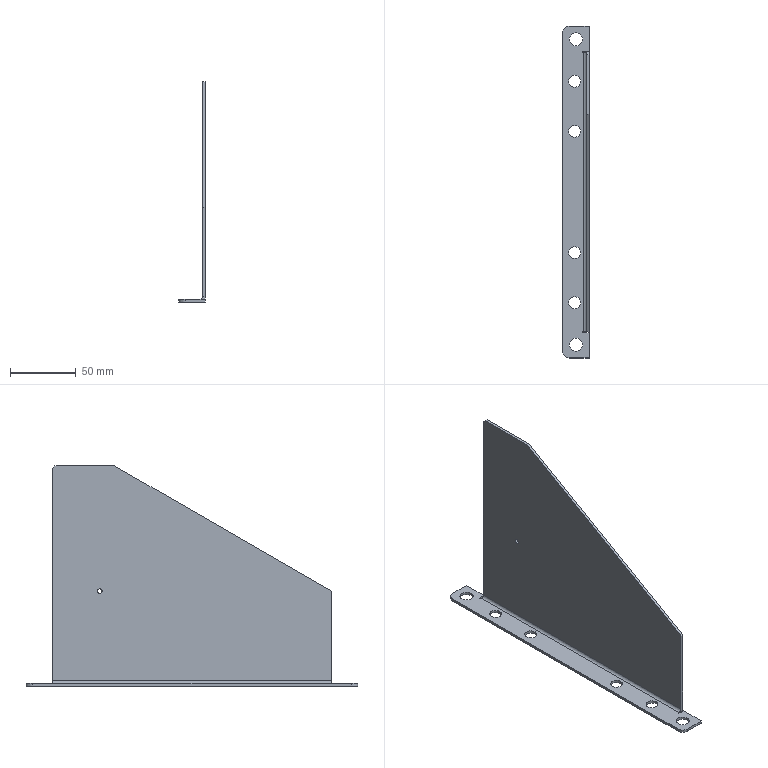Part | STEP file | SYL0380DJ1008_2_7_2_1-3_STEP | 1 solid | 40 faces | box 20 x 252 x 167 mm | volume 62974 mm3 | plane 22 | cylinder 18 | commonest cylinder face diameters 9 x8 10 x6 3.5 x2 4 x1 8 x1
STEP:
#1=CARTESIAN_POINT('',(10.,70.,71.75));
#2=VERTEX_POINT('',#1);
#3=CARTESIAN_POINT('',(8.,70.,71.75));
#4=VERTEX_POINT('',#3);
#5=CARTESIAN_POINT('',(8.,70.,71.75));
#6=DIRECTION('',(-1.,0.,0.));
#7=VECTOR('',#6,1000.);
#8=LINE('',#5,#7);
#9=EDGE_CURVE('',#2,#4,#8,.T.);
#10=ORIENTED_EDGE('',*,*,#9,.F.);
#11=CARTESIAN_POINT('',(10.,70.,68.25));
#12=VERTEX_POINT('',#11);
#13=CARTESIAN_POINT('',(10.,70.,70.));
#14=DIRECTION('',(1.,0.,0.));
#15=DIRECTION('',(0.,0.,-1.));
#16=AXIS2_PLACEMENT_3D('',#13,#14,#15);
#17=CIRCLE('',#16,1.75);
#18=EDGE_CURVE('',#2,#12,#17,.T.);
#19=ORIENTED_EDGE('',*,*,#18,.T.);
#20=CARTESIAN_POINT('',(8.,70.,68.25));
#21=VERTEX_POINT('',#20);
#22=CARTESIAN_POINT('',(8.,70.,68.25));
#23=DIRECTION('',(-1.,0.,0.));
#24=VECTOR('',#23,1000.);
#25=LINE('',#22,#24);
#26=EDGE_CURVE('',#12,#21,#25,.T.);
#27=ORIENTED_EDGE('',*,*,#26,.T.);
#28=CARTESIAN_POINT('',(8.,70.,70.));
#29=DIRECTION('',(1.,0.,0.));
#30=DIRECTION('',(0.,0.,1.));
#31=AXIS2_PLACEMENT_3D('',#28,#29,#30);
#32=CIRCLE('',#31,1.75);
#33=EDGE_CURVE('',#4,#21,#32,.T.);
#34=ORIENTED_EDGE('',*,*,#33,.F.);
#35=EDGE_LOOP('',(#10,#19,#27,#34));
#36=FACE_OUTER_BOUND('',#35,.T.);
#37=CARTESIAN_POINT('',(8.,70.,70.));
#38=DIRECTION('',(-1.,0.,0.));
#39=DIRECTION('',(0.,0.,1.));
#40=AXIS2_PLACEMENT_3D('',#37,#38,#39);
#41=CYLINDRICAL_SURFACE('',#40,1.75);
#42=ADVANCED_FACE('',(#36),#41,.F.);
#43=CARTESIAN_POINT('',(-5.,116.,-2.));
#44=VERTEX_POINT('',#43);
#45=CARTESIAN_POINT('',(-5.,116.,0.));
#46=VERTEX_POINT('',#45);
#47=CARTESIAN_POINT('',(-5.,116.,0.));
#48=DIRECTION('',(0.,0.,1.));
#49=VECTOR('',#48,1000.);
#50=LINE('',#47,#49);
#51=EDGE_CURVE('',#44,#46,#50,.T.);
#52=ORIENTED_EDGE('',*,*,#51,.F.);
#53=CARTESIAN_POINT('',(5.,116.,-2.));
#54=VERTEX_POINT('',#53);
#55=CARTESIAN_POINT('',(0.,116.,-2.));
#56=DIRECTION('',(0.,0.,-1.));
#57=DIRECTION('',(-1.,0.,0.));
#58=AXIS2_PLACEMENT_3D('',#55,#56,#57);
#59=CIRCLE('',#58,5.);
#60=EDGE_CURVE('',#44,#54,#59,.T.);
#61=ORIENTED_EDGE('',*,*,#60,.T.);
#62=CARTESIAN_POINT('',(5.,116.,0.));
#63=VERTEX_POINT('',#62);
#64=CARTESIAN_POINT('',(5.,116.,0.));
#65=DIRECTION('',(0.,0.,1.));
#66=VECTOR('',#65,1000.);
#67=LINE('',#64,#66);
#68=EDGE_CURVE('',#54,#63,#67,.T.);
#69=ORIENTED_EDGE('',*,*,#68,.T.);
#70=CARTESIAN_POINT('',(0.,116.,0.));
#71=DIRECTION('',(0.,0.,-1.));
#72=DIRECTION('',(-1.,0.,0.));
#73=AXIS2_PLACEMENT_3D('',#70,#71,#72);
#74=CIRCLE('',#73,5.);
#75=EDGE_CURVE('',#46,#63,#74,.T.);
#76=ORIENTED_EDGE('',*,*,#75,.F.);
#77=EDGE_LOOP('',(#52,#61,#69,#76));
#78=FACE_OUTER_BOUND('',#77,.T.);
#79=CARTESIAN_POINT('',(0.,116.,0.));
#80=DIRECTION('',(0.,0.,1.));
#81=DIRECTION('',(1.,0.,0.));
#82=AXIS2_PLACEMENT_3D('',#79,#80,#81);
#83=CYLINDRICAL_SURFACE('',#82,5.);
#84=ADVANCED_FACE('',(#78),#83,.F.);
#85=CARTESIAN_POINT('',(-5.,-116.,-2.));
#86=VERTEX_POINT('',#85);
#87=CARTESIAN_POINT('',(-5.,-116.,0.));
#88=VERTEX_POINT('',#87);
#89=CARTESIAN_POINT('',(-5.,-116.,0.));
#90=DIRECTION('',(0.,0.,1.));
#91=VECTOR('',#90,1000.);
#92=LINE('',#89,#91);
#93=EDGE_CURVE('',#86,#88,#92,.T.);
#94=ORIENTED_EDGE('',*,*,#93,.F.);
#95=CARTESIAN_POINT('',(5.,-116.,-2.));
#96=VERTEX_POINT('',#95);
#97=CARTESIAN_POINT('',(0.,-116.,-2.));
#98=DIRECTION('',(0.,0.,-1.));
#99=DIRECTION('',(-1.,0.,0.));
#100=AXIS2_PLACEMENT_3D('',#97,#98,#99);
#101=CIRCLE('',#100,5.);
#102=EDGE_CURVE('',#86,#96,#101,.T.);
#103=ORIENTED_EDGE('',*,*,#102,.T.);
#104=CARTESIAN_POINT('',(5.,-116.,0.));
#105=VERTEX_POINT('',#104);
#106=CARTESIAN_POINT('',(5.,-116.,0.));
#107=DIRECTION('',(0.,0.,1.));
#108=VECTOR('',#107,1000.);
#109=LINE('',#106,#108);
#110=EDGE_CURVE('',#96,#105,#109,.T.);
#111=ORIENTED_EDGE('',*,*,#110,.T.);
#112=CARTESIAN_POINT('',(0.,-116.,0.));
#113=DIRECTION('',(0.,0.,-1.));
#114=DIRECTION('',(-1.,0.,0.));
#115=AXIS2_PLACEMENT_3D('',#112,#113,#114);
#116=CIRCLE('',#115,5.);
#117=EDGE_CURVE('',#88,#105,#116,.T.);
#118=ORIENTED_EDGE('',*,*,#117,.F.);
#119=EDGE_LOOP('',(#94,#103,#111,#118));
#120=FACE_OUTER_BOUND('',#119,.T.);
#121=CARTESIAN_POINT('',(0.,-116.,0.));
#122=DIRECTION('',(0.,0.,1.));
#123=DIRECTION('',(1.,0.,0.));
#124=AXIS2_PLACEMENT_3D('',#121,#122,#123);
#125=CYLINDRICAL_SURFACE('',#124,5.);
#126=ADVANCED_FACE('',(#120),#125,.F.);
#127=CARTESIAN_POINT('',(3.5,-84.,-2.));
#128=VERTEX_POINT('',#127);
#129=CARTESIAN_POINT('',(3.5,-84.,0.));
#130=VERTEX_POINT('',#129);
#131=CARTESIAN_POINT('',(3.5,-84.,0.));
#132=DIRECTION('',(0.,0.,1.));
#133=VECTOR('',#132,1000.);
#134=LINE('',#131,#133);
#135=EDGE_CURVE('',#128,#130,#134,.T.);
#136=ORIENTED_EDGE('',*,*,#135,.F.);
#137=CARTESIAN_POINT('',(-5.5,-84.,-2.));
#138=VERTEX_POINT('',#137);
#139=CARTESIAN_POINT('',(-1.,-84.,-2.));
#140=DIRECTION('',(0.,0.,-1.));
#141=DIRECTION('',(-1.,0.,0.));
#142=AXIS2_PLACEMENT_3D('',#139,#140,#141);
#143=CIRCLE('',#142,4.5);
#144=EDGE_CURVE('',#128,#138,#143,.T.);
#145=ORIENTED_EDGE('',*,*,#144,.T.);
#146=CARTESIAN_POINT('',(-5.5,-84.,0.));
#147=VERTEX_POINT('',#146);
#148=CARTESIAN_POINT('',(-5.5,-84.,0.));
#149=DIRECTION('',(0.,0.,1.));
#150=VECTOR('',#149,1000.);
#151=LINE('',#148,#150);
#152=EDGE_CURVE('',#138,#147,#151,.T.);
#153=ORIENTED_EDGE('',*,*,#152,.T.);
#154=CARTESIAN_POINT('',(-1.,-84.,0.));
#155=DIRECTION('',(0.,0.,-1.));
#156=DIRECTION('',(1.,0.,0.));
#157=AXIS2_PLACEMENT_3D('',#154,#155,#156);
#158=CIRCLE('',#157,4.5);
#159=EDGE_CURVE('',#130,#147,#158,.T.);
#160=ORIENTED_EDGE('',*,*,#159,.F.);
#161=EDGE_LOOP('',(#136,#145,#153,#160));
#162=FACE_OUTER_BOUND('',#161,.T.);
#163=CARTESIAN_POINT('',(-1.,-84.,0.));
#164=DIRECTION('',(0.,0.,1.));
#165=DIRECTION('',(1.,0.,0.));
#166=AXIS2_PLACEMENT_3D('',#163,#164,#165);
#167=CYLINDRICAL_SURFACE('',#166,4.5);
#168=ADVANCED_FACE('',(#162),#167,.F.);
#169=CARTESIAN_POINT('',(3.5,-46.,-2.));
#170=VERTEX_POINT('',#169);
#171=CARTESIAN_POINT('',(3.5,-46.,0.));
#172=VERTEX_POINT('',#171);
#173=CARTESIAN_POINT('',(3.5,-46.,0.));
#174=DIRECTION('',(0.,0.,1.));
#175=VECTOR('',#174,1000.);
#176=LINE('',#173,#175);
#177=EDGE_CURVE('',#170,#172,#176,.T.);
#178=ORIENTED_EDGE('',*,*,#177,.F.);
#179=CARTESIAN_POINT('',(-5.5,-46.,-2.));
#180=VERTEX_POINT('',#179);
#181=CARTESIAN_POINT('',(-1.,-46.,-2.));
#182=DIRECTION('',(0.,0.,-1.));
#183=DIRECTION('',(-1.,0.,0.));
#184=AXIS2_PLACEMENT_3D('',#181,#182,#183);
#185=CIRCLE('',#184,4.5);
#186=EDGE_CURVE('',#170,#180,#185,.T.);
#187=ORIENTED_EDGE('',*,*,#186,.T.);
#188=CARTESIAN_POINT('',(-5.5,-46.,0.));
#189=VERTEX_POINT('',#188);
#190=CARTESIAN_POINT('',(-5.5,-46.,0.));
#191=DIRECTION('',(0.,0.,1.));
#192=VECTOR('',#191,1000.);
#193=LINE('',#190,#192);
#194=EDGE_CURVE('',#180,#189,#193,.T.);
#195=ORIENTED_EDGE('',*,*,#194,.T.);
#196=CARTESIAN_POINT('',(-1.,-46.,0.));
#197=DIRECTION('',(0.,0.,-1.));
#198=DIRECTION('',(1.,0.,0.));
#199=AXIS2_PLACEMENT_3D('',#196,#197,#198);
#200=CIRCLE('',#199,4.5);
#201=EDGE_CURVE('',#172,#189,#200,.T.);
#202=ORIENTED_EDGE('',*,*,#201,.F.);
#203=EDGE_LOOP('',(#178,#187,#195,#202));
#204=FACE_OUTER_BOUND('',#203,.T.);
#205=CARTESIAN_POINT('',(-1.,-46.,0.));
#206=DIRECTION('',(0.,0.,1.));
#207=DIRECTION('',(1.,0.,0.));
#208=AXIS2_PLACEMENT_3D('',#205,#206,#207);
#209=CYLINDRICAL_SURFACE('',#208,4.5);
#210=ADVANCED_FACE('',(#204),#209,.F.);
#211=CARTESIAN_POINT('',(3.5,46.,-2.));
#212=VERTEX_POINT('',#211);
#213=CARTESIAN_POINT('',(3.5,46.,0.));
#214=VERTEX_POINT('',#213);
#215=CARTESIAN_POINT('',(3.5,46.,0.));
#216=DIRECTION('',(0.,0.,1.));
#217=VECTOR('',#216,1000.);
#218=LINE('',#215,#217);
#219=EDGE_CURVE('',#212,#214,#218,.T.);
#220=ORIENTED_EDGE('',*,*,#219,.F.);
#221=CARTESIAN_POINT('',(-5.5,46.,-2.));
#222=VERTEX_POINT('',#221);
#223=CARTESIAN_POINT('',(-1.,46.,-2.));
#224=DIRECTION('',(0.,0.,-1.));
#225=DIRECTION('',(-1.,0.,0.));
#226=AXIS2_PLACEMENT_3D('',#223,#224,#225);
#227=CIRCLE('',#226,4.5);
#228=EDGE_CURVE('',#212,#222,#227,.T.);
#229=ORIENTED_EDGE('',*,*,#228,.T.);
#230=CARTESIAN_POINT('',(-5.5,46.,0.));
#231=VERTEX_POINT('',#230);
#232=CARTESIAN_POINT('',(-5.5,46.,0.));
#233=DIRECTION('',(0.,0.,1.));
#234=VECTOR('',#233,1000.);
#235=LINE('',#232,#234);
#236=EDGE_CURVE('',#222,#231,#235,.T.);
#237=ORIENTED_EDGE('',*,*,#236,.T.);
#238=CARTESIAN_POINT('',(-1.,46.,0.));
#239=DIRECTION('',(0.,0.,-1.));
#240=DIRECTION('',(1.,0.,0.));
#241=AXIS2_PLACEMENT_3D('',#238,#239,#240);
#242=CIRCLE('',#241,4.5);
#243=EDGE_CURVE('',#214,#231,#242,.T.);
#244=ORIENTED_EDGE('',*,*,#243,.F.);
#245=EDGE_LOOP('',(#220,#229,#237,#244));
#246=FACE_OUTER_BOUND('',#245,.T.);
#247=CARTESIAN_POINT('',(-1.,46.,0.));
#248=DIRECTION('',(0.,0.,1.));
#249=DIRECTION('',(1.,0.,0.));
#250=AXIS2_PLACEMENT_3D('',#247,#248,#249);
#251=CYLINDRICAL_SURFACE('',#250,4.5);
#252=ADVANCED_FACE('',(#246),#251,.F.);
#253=CARTESIAN_POINT('',(3.5,84.,-2.));
#254=VERTEX_POINT('',#253);
#255=CARTESIAN_POINT('',(3.5,84.,0.));
#256=VERTEX_POINT('',#255);
#257=CARTESIAN_POINT('',(3.5,84.,0.));
#258=DIRECTION('',(0.,0.,1.));
#259=VECTOR('',#258,1000.);
#260=LINE('',#257,#259);
#261=EDGE_CURVE('',#254,#256,#260,.T.);
#262=ORIENTED_EDGE('',*,*,#261,.F.);
#263=CARTESIAN_POINT('',(-5.5,84.,-2.));
#264=VERTEX_POINT('',#263);
#265=CARTESIAN_POINT('',(-1.,84.,-2.));
#266=DIRECTION('',(0.,0.,-1.));
#267=DIRECTION('',(-1.,0.,0.));
#268=AXIS2_PLACEMENT_3D('',#265,#266,#267);
#269=CIRCLE('',#268,4.5);
#270=EDGE_CURVE('',#254,#264,#269,.T.);
#271=ORIENTED_EDGE('',*,*,#270,.T.);
#272=CARTESIAN_POINT('',(-5.5,84.,0.));
#273=VERTEX_POINT('',#272);
#274=CARTESIAN_POINT('',(-5.5,84.,0.));
#275=DIRECTION('',(0.,0.,1.));
#276=VECTOR('',#275,1000.);
#277=LINE('',#274,#276);
#278=EDGE_CURVE('',#264,#273,#277,.T.);
#279=ORIENTED_EDGE('',*,*,#278,.T.);
#280=CARTESIAN_POINT('',(-1.,84.,0.));
#281=DIRECTION('',(0.,0.,-1.));
#282=DIRECTION('',(1.,0.,0.));
#283=AXIS2_PLACEMENT_3D('',#280,#281,#282);
#284=CIRCLE('',#283,4.5);
#285=EDGE_CURVE('',#256,#273,#284,.T.);
#286=ORIENTED_EDGE('',*,*,#285,.F.);
#287=EDGE_LOOP('',(#262,#271,#279,#286));
#288=FACE_OUTER_BOUND('',#287,.T.);
#289=CARTESIAN_POINT('',(-1.,84.,0.));
#290=DIRECTION('',(0.,0.,1.));
#291=DIRECTION('',(1.,0.,0.));
#292=AXIS2_PLACEMENT_3D('',#289,#290,#291);
#293=CYLINDRICAL_SURFACE('',#292,4.5);
#294=ADVANCED_FACE('',(#288),#293,.F.);
#295=CARTESIAN_POINT('',(10.,-106.,70.));
#296=VERTEX_POINT('',#295);
#297=CARTESIAN_POINT('',(8.,-106.,70.));
#298=VERTEX_POINT('',#297);
#299=CARTESIAN_POINT('',(8.,-106.,70.));
#300=DIRECTION('',(-1.,0.,0.));
#301=VECTOR('',#300,1000.);
#302=LINE('',#299,#301);
#303=EDGE_CURVE('',#296,#298,#302,.T.);
#304=ORIENTED_EDGE('',*,*,#303,.F.);
#305=CARTESIAN_POINT('',(10.,58.545,165.));
#306=VERTEX_POINT('',#305);
#307=CARTESIAN_POINT('',(10.,-106.,70.));
#308=DIRECTION('',(0.,0.866,0.5));
#309=VECTOR('',#308,1000.);
#310=LINE('',#307,#309);
#311=EDGE_CURVE('',#296,#306,#310,.T.);
#312=ORIENTED_EDGE('',*,*,#311,.T.);
#313=CARTESIAN_POINT('',(8.,58.545,165.));
#314=VERTEX_POINT('',#313);
#315=CARTESIAN_POINT('',(8.,58.545,165.));
#316=DIRECTION('',(-1.,0.,0.));
#317=VECTOR('',#316,1000.);
#318=LINE('',#315,#317);
#319=EDGE_CURVE('',#306,#314,#318,.T.);
#320=ORIENTED_EDGE('',*,*,#319,.T.);
#321=CARTESIAN_POINT('',(8.,-106.,70.));
#322=DIRECTION('',(0.,0.866,0.5));
#323=VECTOR('',#322,1000.);
#324=LINE('',#321,#323);
#325=EDGE_CURVE('',#298,#314,#324,.T.);
#326=ORIENTED_EDGE('',*,*,#325,.F.);
#327=EDGE_LOOP('',(#304,#312,#320,#326));
#328=FACE_OUTER_BOUND('',#327,.T.);
#329=CARTESIAN_POINT('',(8.,-106.,70.));
#330=DIRECTION('',(0.,-0.5,0.866));
#331=DIRECTION('',(0.,0.866,0.5));
#332=AXIS2_PLACEMENT_3D('',#329,#330,#331);
#333=PLANE('',#332);
#334=ADVANCED_FACE('',(#328),#333,.T.);
#335=ORIENTED_EDGE('',*,*,#319,.F.);
#336=CARTESIAN_POINT('',(10.,104.,165.));
#337=VERTEX_POINT('',#336);
#338=CARTESIAN_POINT('',(10.,-66.125,165.));
#339=DIRECTION('',(0.,-1.,0.));
#340=VECTOR('',#339,1000.);
#341=LINE('',#338,#340);
#342=EDGE_CURVE('',#337,#306,#341,.T.);
#343=ORIENTED_EDGE('',*,*,#342,.F.);
#344=CARTESIAN_POINT('',(8.,104.,165.));
#345=VERTEX_POINT('',#344);
#346=CARTESIAN_POINT('',(8.,104.,165.));
#347=DIRECTION('',(-1.,0.,0.));
#348=VECTOR('',#347,1000.);
#349=LINE('',#346,#348);
#350=EDGE_CURVE('',#337,#345,#349,.T.);
#351=ORIENTED_EDGE('',*,*,#350,.T.);
#352=CARTESIAN_POINT('',(8.,104.,165.));
#353=DIRECTION('',(0.,-1.,0.));
#354=VECTOR('',#353,1000.);
#355=LINE('',#352,#354);
#356=EDGE_CURVE('',#345,#314,#355,.T.);
#357=ORIENTED_EDGE('',*,*,#356,.T.);
#358=EDGE_LOOP('',(#335,#343,#351,#357));
#359=FACE_OUTER_BOUND('',#358,.T.);
#360=CARTESIAN_POINT('',(8.,104.,165.));
#361=DIRECTION('',(0.,0.,-1.));
#362=DIRECTION('',(0.,-1.,0.));
#363=AXIS2_PLACEMENT_3D('',#360,#361,#362);
#364=PLANE('',#363);
#365=ADVANCED_FACE('',(#359),#364,.F.);
#366=ORIENTED_EDGE('',*,*,#350,.F.);
#367=CARTESIAN_POINT('',(10.,106.,163.));
#368=VERTEX_POINT('',#367);
#369=CARTESIAN_POINT('',(10.,104.,165.));
#370=DIRECTION('',(0.,0.7071,-0.7071));
#371=VECTOR('',#370,1000.);
#372=LINE('',#369,#371);
#373=EDGE_CURVE('',#337,#368,#372,.T.);
#374=ORIENTED_EDGE('',*,*,#373,.T.);
#375=CARTESIAN_POINT('',(8.,106.,163.));
#376=VERTEX_POINT('',#375);
#377=CARTESIAN_POINT('',(8.,106.,163.));
#378=DIRECTION('',(-1.,0.,0.));
#379=VECTOR('',#378,1000.);
#380=LINE('',#377,#379);
#381=EDGE_CURVE('',#368,#376,#380,.T.);
#382=ORIENTED_EDGE('',*,*,#381,.T.);
#383=CARTESIAN_POINT('',(8.,104.,165.));
#384=DIRECTION('',(0.,0.7071,-0.7071));
#385=VECTOR('',#384,1000.);
#386=LINE('',#383,#385);
#387=EDGE_CURVE('',#345,#376,#386,.T.);
#388=ORIENTED_EDGE('',*,*,#387,.F.);
#389=EDGE_LOOP('',(#366,#374,#382,#388));
#390=FACE_OUTER_BOUND('',#389,.T.);
#391=CARTESIAN_POINT('',(8.,104.,165.));
#392=DIRECTION('',(0.,0.7071,0.7071));
#393=DIRECTION('',(0.,0.7071,-0.7071));
#394=AXIS2_PLACEMENT_3D('',#391,#392,#393);
#395=PLANE('',#394);
#396=ADVANCED_FACE('',(#390),#395,.T.);
#397=ORIENTED_EDGE('',*,*,#381,.F.);
#398=CARTESIAN_POINT('',(10.,106.,2.));
#399=VERTEX_POINT('',#398);
#400=CARTESIAN_POINT('',(10.,106.,-2.));
#401=DIRECTION('',(0.,0.,1.));
#402=VECTOR('',#401,1000.);
#403=LINE('',#400,#402);
#404=EDGE_CURVE('',#399,#368,#403,.T.);
#405=ORIENTED_EDGE('',*,*,#404,.F.);
#406=CARTESIAN_POINT('',(8.,106.,2.));
#407=VERTEX_POINT('',#406);
#408=CARTESIAN_POINT('',(8.,106.,2.));
#409=DIRECTION('',(-1.,0.,0.));
#410=VECTOR('',#409,1000.);
#411=LINE('',#408,#410);
#412=EDGE_CURVE('',#399,#407,#411,.T.);
#413=ORIENTED_EDGE('',*,*,#412,.T.);
#414=CARTESIAN_POINT('',(8.,106.,2.));
#415=DIRECTION('',(0.,0.,1.));
#416=VECTOR('',#415,1000.);
#417=LINE('',#414,#416);
#418=EDGE_CURVE('',#407,#376,#417,.T.);
#419=ORIENTED_EDGE('',*,*,#418,.T.);
#420=EDGE_LOOP('',(#397,#405,#413,#419));
#421=FACE_OUTER_BOUND('',#420,.T.);
#422=CARTESIAN_POINT('',(8.,106.,2.));
#423=DIRECTION('',(0.,-1.,0.));
#424=DIRECTION('',(0.,0.,1.));
#425=AXIS2_PLACEMENT_3D('',#422,#423,#424);
#426=PLANE('',#425);
#427=ADVANCED_FACE('',(#421),#426,.F.);
#428=ORIENTED_EDGE('',*,*,#412,.F.);
#429=CARTESIAN_POINT('',(6.,106.,-2.));
#430=VERTEX_POINT('',#429);
#431=CARTESIAN_POINT('',(6.,106.,2.));
#432=DIRECTION('',(0.,-1.,0.));
#433=DIRECTION('',(0.,0.,1.));
#434=AXIS2_PLACEMENT_3D('',#431,#432,#433);
#435=CIRCLE('',#434,4.);
#436=EDGE_CURVE('',#430,#399,#435,.T.);
#437=ORIENTED_EDGE('',*,*,#436,.F.);
#438=CARTESIAN_POINT('',(6.,106.,0.));
#439=VERTEX_POINT('',#438);
#440=CARTESIAN_POINT('',(6.,106.,0.));
#441=DIRECTION('',(0.,0.,1.));
#442=VECTOR('',#441,1000.);
#443=LINE('',#440,#442);
#444=EDGE_CURVE('',#430,#439,#443,.T.);
#445=ORIENTED_EDGE('',*,*,#444,.T.);
#446=CARTESIAN_POINT('',(6.,106.,2.));
#447=DIRECTION('',(0.,-1.,0.));
#448=DIRECTION('',(0.,0.,-1.));
#449=AXIS2_PLACEMENT_3D('',#446,#447,#448);
#450=CIRCLE('',#449,2.);
#451=EDGE_CURVE('',#439,#407,#450,.T.);
#452=ORIENTED_EDGE('',*,*,#451,.T.);
#453=EDGE_LOOP('',(#428,#437,#445,#452));
#454=FACE_OUTER_BOUND('',#453,.T.);
#455=CARTESIAN_POINT('',(6.,106.,2.));
#456=DIRECTION('',(0.,1.,0.));
#457=DIRECTION('',(0.,0.,1.));
#458=AXIS2_PLACEMENT_3D('',#455,#456,#457);
#459=PLANE('',#458);
#460=ADVANCED_FACE('',(#454),#459,.T.);
#461=ORIENTED_EDGE('',*,*,#444,.F.);
#462=CARTESIAN_POINT('',(5.,106.,-2.));
#463=VERTEX_POINT('',#462);
#464=CARTESIAN_POINT('',(0.,106.,-2.));
#465=DIRECTION('',(1.,0.,0.));
#466=VECTOR('',#465,1000.);
#467=LINE('',#464,#466);
#468=EDGE_CURVE('',#463,#430,#467,.T.);
#469=ORIENTED_EDGE('',*,*,#468,.F.);
#470=CARTESIAN_POINT('',(5.,106.,0.));
#471=VERTEX_POINT('',#470);
#472=CARTESIAN_POINT('',(5.,106.,0.));
#473=DIRECTION('',(0.,0.,1.));
#474=VECTOR('',#473,1000.);
#475=LINE('',#472,#474);
#476=EDGE_CURVE('',#463,#471,#475,.T.);
#477=ORIENTED_EDGE('',*,*,#476,.T.);
#478=CARTESIAN_POINT('',(0.,106.,0.));
#479=DIRECTION('',(1.,0.,0.));
#480=VECTOR('',#479,1000.);
#481=LINE('',#478,#480);
#482=EDGE_CURVE('',#471,#439,#481,.T.);
#483=ORIENTED_EDGE('',*,*,#482,.T.);
#484=EDGE_LOOP('',(#461,#469,#477,#483));
#485=FACE_OUTER_BOUND('',#484,.T.);
#486=CARTESIAN_POINT('',(0.,106.,0.));
#487=DIRECTION('',(0.,-1.,0.));
#488=DIRECTION('',(1.,0.,0.));
#489=AXIS2_PLACEMENT_3D('',#486,#487,#488);
#490=PLANE('',#489);
#491=ADVANCED_FACE('',(#485),#490,.F.);
#492=ORIENTED_EDGE('',*,*,#476,.F.);
#493=CARTESIAN_POINT('',(5.,107.,-2.));
#494=VERTEX_POINT('',#493);
#495=CARTESIAN_POINT('',(5.,0.,-2.));
#496=DIRECTION('',(0.,-1.,0.));
#497=VECTOR('',#496,1000.);
#498=LINE('',#495,#497);
#499=EDGE_CURVE('',#494,#463,#498,.T.);
#500=ORIENTED_EDGE('',*,*,#499,.F.);
#501=CARTESIAN_POINT('',(5.,107.,0.));
#502=VERTEX_POINT('',#501);
#503=CARTESIAN_POINT('',(5.,107.,0.));
#504=DIRECTION('',(0.,0.,1.));
#505=VECTOR('',#504,1000.);
#506=LINE('',#503,#505);
#507=EDGE_CURVE('',#494,#502,#506,.T.);
#508=ORIENTED_EDGE('',*,*,#507,.T.);
#509=CARTESIAN_POINT('',(5.,0.,0.));
#510=DIRECTION('',(0.,-1.,0.));
#511=VECTOR('',#510,1000.);
#512=LINE('',#509,#511);
#513=EDGE_CURVE('',#502,#471,#512,.T.);
#514=ORIENTED_EDGE('',*,*,#513,.T.);
#515=EDGE_LOOP('',(#492,#500,#508,#514));
#516=FACE_OUTER_BOUND('',#515,.T.);
#517=CARTESIAN_POINT('',(5.,0.,0.));
#518=DIRECTION('',(-1.,0.,0.));
#519=DIRECTION('',(0.,-1.,0.));
#520=AXIS2_PLACEMENT_3D('',#517,#518,#519);
#521=PLANE('',#520);
#522=ADVANCED_FACE('',(#516),#521,.F.);
#523=ORIENTED_EDGE('',*,*,#507,.F.);
#524=CARTESIAN_POINT('',(10.,107.,-2.));
#525=VERTEX_POINT('',#524);
#526=CARTESIAN_POINT('',(0.,107.,-2.));
#527=DIRECTION('',(-1.,0.,0.));
#528=VECTOR('',#527,1000.);
#529=LINE('',#526,#528);
#530=EDGE_CURVE('',#525,#494,#529,.T.);
#531=ORIENTED_EDGE('',*,*,#530,.F.);
#532=CARTESIAN_POINT('',(10.,107.,0.));
#533=VERTEX_POINT('',#532);
#534=CARTESIAN_POINT('',(10.,107.,0.));
#535=DIRECTION('',(0.,0.,1.));
#536=VECTOR('',#535,1000.);
#537=LINE('',#534,#536);
#538=EDGE_CURVE('',#525,#533,#537,.T.);
#539=ORIENTED_EDGE('',*,*,#538,.T.);
#540=CARTESIAN_POINT('',(0.,107.,0.));
#541=DIRECTION('',(-1.,0.,0.));
#542=VECTOR('',#541,1000.);
#543=LINE('',#540,#542);
#544=EDGE_CURVE('',#533,#502,#543,.T.);
#545=ORIENTED_EDGE('',*,*,#544,.T.);
#546=EDGE_LOOP('',(#523,#531,#539,#545));
#547=FACE_OUTER_BOUND('',#546,.T.);
#548=CARTESIAN_POINT('',(0.,107.,0.));
#549=DIRECTION('',(0.,1.,0.));
#550=DIRECTION('',(-1.,0.,0.));
#551=AXIS2_PLACEMENT_3D('',#548,#549,#550);
#552=PLANE('',#551);
#553=ADVANCED_FACE('',(#547),#552,.F.);
#554=ORIENTED_EDGE('',*,*,#538,.F.);
#555=CARTESIAN_POINT('',(10.,126.,-2.));
#556=VERTEX_POINT('',#555);
#557=CARTESIAN_POINT('',(10.,0.,-2.));
#558=DIRECTION('',(0.,1.,0.));
#559=VECTOR('',#558,1000.);
#560=LINE('',#557,#559);
#561=EDGE_CURVE('',#525,#556,#560,.T.);
#562=ORIENTED_EDGE('',*,*,#561,.T.);
#563=CARTESIAN_POINT('',(10.,126.,0.));
#564=VERTEX_POINT('',#563);
#565=CARTESIAN_POINT('',(10.,126.,0.));
#566=DIRECTION('',(0.,0.,1.));
#567=VECTOR('',#566,1000.);
#568=LINE('',#565,#567);
#569=EDGE_CURVE('',#556,#564,#568,.T.);
#570=ORIENTED_EDGE('',*,*,#569,.T.);
#571=CARTESIAN_POINT('',(10.,106.,0.));
#572=DIRECTION('',(0.,1.,0.));
#573=VECTOR('',#572,1000.);
#574=LINE('',#571,#573);
#575=EDGE_CURVE('',#533,#564,#574,.T.);
#576=ORIENTED_EDGE('',*,*,#575,.F.);
#577=EDGE_LOOP('',(#554,#562,#570,#576));
#578=FACE_OUTER_BOUND('',#577,.T.);
#579=CARTESIAN_POINT('',(10.,106.,0.));
#580=DIRECTION('',(1.,0.,0.));
#581=DIRECTION('',(0.,1.,0.));
#582=AXIS2_PLACEMENT_3D('',#579,#580,#581);
#583=PLANE('',#582);
#584=ADVANCED_FACE('',(#578),#583,.T.);
#585=ORIENTED_EDGE('',*,*,#569,.F.);
#586=CARTESIAN_POINT('',(-5.,126.,-2.));
#587=VERTEX_POINT('',#586);
#588=CARTESIAN_POINT('',(0.,126.,-2.));
#589=DIRECTION('',(-1.,0.,0.));
#590=VECTOR('',#589,1000.);
#591=LINE('',#588,#590);
#592=EDGE_CURVE('',#556,#587,#591,.T.);
#593=ORIENTED_EDGE('',*,*,#592,.T.);
#594=CARTESIAN_POINT('',(-5.,126.,0.));
#595=VERTEX_POINT('',#594);
#596=CARTESIAN_POINT('',(-5.,126.,0.));
#597=DIRECTION('',(0.,0.,1.));
#598=VECTOR('',#597,1000.);
#599=LINE('',#596,#598);
#600=EDGE_CURVE('',#587,#595,#599,.T.);
#601=ORIENTED_EDGE('',*,*,#600,.T.);
#602=CARTESIAN_POINT('',(10.,126.,0.));
#603=DIRECTION('',(-1.,0.,0.));
#604=VECTOR('',#603,1000.);
#605=LINE('',#602,#604);
#606=EDGE_CURVE('',#564,#595,#605,.T.);
#607=ORIENTED_EDGE('',*,*,#606,.F.);
#608=EDGE_LOOP('',(#585,#593,#601,#607));
#609=FACE_OUTER_BOUND('',#608,.T.);
#610=CARTESIAN_POINT('',(10.,126.,0.));
#611=DIRECTION('',(0.,1.,0.));
#612=DIRECTION('',(-1.,0.,0.));
#613=AXIS2_PLACEMENT_3D('',#610,#611,#612);
#614=PLANE('',#613);
#615=ADVANCED_FACE('',(#609),#614,.T.);
#616=ORIENTED_EDGE('',*,*,#600,.F.);
#617=CARTESIAN_POINT('',(-10.,121.,-2.));
#618=VERTEX_POINT('',#617);
#619=CARTESIAN_POINT('',(-5.,121.,-2.));
#620=DIRECTION('',(0.,0.,1.));
#621=DIRECTION('',(1.,0.,0.));
#622=AXIS2_PLACEMENT_3D('',#619,#620,#621);
#623=CIRCLE('',#622,5.);
#624=EDGE_CURVE('',#587,#618,#623,.T.);
#625=ORIENTED_EDGE('',*,*,#624,.T.);
#626=CARTESIAN_POINT('',(-10.,121.,0.));
#627=VERTEX_POINT('',#626);
#628=CARTESIAN_POINT('',(-10.,121.,0.));
#629=DIRECTION('',(0.,0.,1.));
#630=VECTOR('',#629,1000.);
#631=LINE('',#628,#630);
#632=EDGE_CURVE('',#618,#627,#631,.T.);
#633=ORIENTED_EDGE('',*,*,#632,.T.);
#634=CARTESIAN_POINT('',(-5.,121.,0.));
#635=DIRECTION('',(0.,0.,1.));
#636=DIRECTION('',(0.,1.,0.));
#637=AXIS2_PLACEMENT_3D('',#634,#635,#636);
#638=CIRCLE('',#637,5.);
#639=EDGE_CURVE('',#595,#627,#638,.T.);
#640=ORIENTED_EDGE('',*,*,#639,.F.);
#641=EDGE_LOOP('',(#616,#625,#633,#640));
#642=FACE_OUTER_BOUND('',#641,.T.);
#643=CARTESIAN_POINT('',(-5.,121.,0.));
#644=DIRECTION('',(0.,0.,1.));
#645=DIRECTION('',(1.,0.,0.));
#646=AXIS2_PLACEMENT_3D('',#643,#644,#645);
#647=CYLINDRICAL_SURFACE('',#646,5.);
#648=ADVANCED_FACE('',(#642),#647,.T.);
#649=ORIENTED_EDGE('',*,*,#632,.F.);
#650=CARTESIAN_POINT('',(-10.,-121.,-2.));
#651=VERTEX_POINT('',#650);
#652=CARTESIAN_POINT('',(-10.,0.,-2.));
#653=DIRECTION('',(0.,-1.,0.));
#654=VECTOR('',#653,1000.);
#655=LINE('',#652,#654);
#656=EDGE_CURVE('',#618,#651,#655,.T.);
#657=ORIENTED_EDGE('',*,*,#656,.T.);
#658=CARTESIAN_POINT('',(-10.,-121.,0.));
#659=VERTEX_POINT('',#658);
#660=CARTESIAN_POINT('',(-10.,-121.,0.));
#661=DIRECTION('',(0.,0.,1.));
#662=VECTOR('',#661,1000.);
#663=LINE('',#660,#662);
#664=EDGE_CURVE('',#651,#659,#663,.T.);
#665=ORIENTED_EDGE('',*,*,#664,.T.);
#666=CARTESIAN_POINT('',(-10.,121.,0.));
#667=DIRECTION('',(0.,-1.,0.));
#668=VECTOR('',#667,1000.);
#669=LINE('',#666,#668);
#670=EDGE_CURVE('',#627,#659,#669,.T.);
#671=ORIENTED_EDGE('',*,*,#670,.F.);
#672=EDGE_LOOP('',(#649,#657,#665,#671));
#673=FACE_OUTER_BOUND('',#672,.T.);
#674=CARTESIAN_POINT('',(-10.,121.,0.));
#675=DIRECTION('',(-1.,0.,0.));
#676=DIRECTION('',(0.,-1.,0.));
#677=AXIS2_PLACEMENT_3D('',#674,#675,#676);
#678=PLANE('',#677);
#679=ADVANCED_FACE('',(#673),#678,.T.);
#680=ORIENTED_EDGE('',*,*,#664,.F.);
#681=CARTESIAN_POINT('',(-5.,-126.,-2.));
#682=VERTEX_POINT('',#681);
#683=CARTESIAN_POINT('',(-5.,-121.,-2.));
#684=DIRECTION('',(0.,0.,1.));
#685=DIRECTION('',(1.,0.,0.));
#686=AXIS2_PLACEMENT_3D('',#683,#684,#685);
#687=CIRCLE('',#686,5.);
#688=EDGE_CURVE('',#651,#682,#687,.T.);
#689=ORIENTED_EDGE('',*,*,#688,.T.);
#690=CARTESIAN_POINT('',(-5.,-126.,0.));
#691=VERTEX_POINT('',#690);
#692=CARTESIAN_POINT('',(-5.,-126.,0.));
#693=DIRECTION('',(0.,0.,1.));
#694=VECTOR('',#693,1000.);
#695=LINE('',#692,#694);
#696=EDGE_CURVE('',#682,#691,#695,.T.);
#697=ORIENTED_EDGE('',*,*,#696,.T.);
#698=CARTESIAN_POINT('',(-5.,-121.,0.));
#699=DIRECTION('',(0.,0.,1.));
#700=DIRECTION('',(-1.,0.,0.));
#701=AXIS2_PLACEMENT_3D('',#698,#699,#700);
#702=CIRCLE('',#701,5.);
#703=EDGE_CURVE('',#659,#691,#702,.T.);
#704=ORIENTED_EDGE('',*,*,#703,.F.);
#705=EDGE_LOOP('',(#680,#689,#697,#704));
#706=FACE_OUTER_BOUND('',#705,.T.);
#707=CARTESIAN_POINT('',(-5.,-121.,0.));
#708=DIRECTION('',(0.,0.,1.));
#709=DIRECTION('',(1.,0.,0.));
#710=AXIS2_PLACEMENT_3D('',#707,#708,#709);
#711=CYLINDRICAL_SURFACE('',#710,5.);
#712=ADVANCED_FACE('',(#706),#711,.T.);
#713=ORIENTED_EDGE('',*,*,#696,.F.);
#714=CARTESIAN_POINT('',(10.,-126.,-2.));
#715=VERTEX_POINT('',#714);
#716=CARTESIAN_POINT('',(0.,-126.,-2.));
#717=DIRECTION('',(1.,0.,0.));
#718=VECTOR('',#717,1000.);
#719=LINE('',#716,#718);
#720=EDGE_CURVE('',#682,#715,#719,.T.);
#721=ORIENTED_EDGE('',*,*,#720,.T.);
#722=CARTESIAN_POINT('',(10.,-126.,0.));
#723=VERTEX_POINT('',#722);
#724=CARTESIAN_POINT('',(10.,-126.,0.));
#725=DIRECTION('',(0.,0.,1.));
#726=VECTOR('',#725,1000.);
#727=LINE('',#724,#726);
#728=EDGE_CURVE('',#715,#723,#727,.T.);
#729=ORIENTED_EDGE('',*,*,#728,.T.);
#730=CARTESIAN_POINT('',(-5.,-126.,0.));
#731=DIRECTION('',(1.,0.,0.));
#732=VECTOR('',#731,1000.);
#733=LINE('',#730,#732);
#734=EDGE_CURVE('',#691,#723,#733,.T.);
#735=ORIENTED_EDGE('',*,*,#734,.F.);
#736=EDGE_LOOP('',(#713,#721,#729,#735));
#737=FACE_OUTER_BOUND('',#736,.T.);
#738=CARTESIAN_POINT('',(-5.,-126.,0.));
#739=DIRECTION('',(0.,-1.,0.));
#740=DIRECTION('',(1.,0.,0.));
#741=AXIS2_PLACEMENT_3D('',#738,#739,#740);
#742=PLANE('',#741);
#743=ADVANCED_FACE('',(#737),#742,.T.);
#744=ORIENTED_EDGE('',*,*,#728,.F.);
#745=CARTESIAN_POINT('',(10.,-107.,-2.));
#746=VERTEX_POINT('',#745);
#747=CARTESIAN_POINT('',(10.,0.,-2.));
#748=DIRECTION('',(0.,1.,0.));
#749=VECTOR('',#748,1000.);
#750=LINE('',#747,#749);
#751=EDGE_CURVE('',#715,#746,#750,.T.);
#752=ORIENTED_EDGE('',*,*,#751,.T.);
#753=CARTESIAN_POINT('',(10.,-107.,0.));
#754=VERTEX_POINT('',#753);
#755=CARTESIAN_POINT('',(10.,-107.,0.));
#756=DIRECTION('',(0.,0.,1.));
#757=VECTOR('',#756,1000.);
#758=LINE('',#755,#757);
#759=EDGE_CURVE('',#746,#754,#758,.T.);
#760=ORIENTED_EDGE('',*,*,#759,.T.);
#761=CARTESIAN_POINT('',(10.,-126.,0.));
#762=DIRECTION('',(0.,1.,0.));
#763=VECTOR('',#762,1000.);
#764=LINE('',#761,#763);
#765=EDGE_CURVE('',#723,#754,#764,.T.);
#766=ORIENTED_EDGE('',*,*,#765,.F.);
#767=EDGE_LOOP('',(#744,#752,#760,#766));
#768=FACE_OUTER_BOUND('',#767,.T.);
#769=CARTESIAN_POINT('',(10.,-126.,0.));
#770=DIRECTION('',(1.,0.,0.));
#771=DIRECTION('',(0.,1.,0.));
#772=AXIS2_PLACEMENT_3D('',#769,#770,#771);
#773=PLANE('',#772);
#774=ADVANCED_FACE('',(#768),#773,.T.);
#775=ORIENTED_EDGE('',*,*,#759,.F.);
#776=CARTESIAN_POINT('',(5.,-107.,-2.));
#777=VERTEX_POINT('',#776);
#778=CARTESIAN_POINT('',(0.,-107.,-2.));
#779=DIRECTION('',(1.,0.,0.));
#780=VECTOR('',#779,1000.);
#781=LINE('',#778,#780);
#782=EDGE_CURVE('',#777,#746,#781,.T.);
#783=ORIENTED_EDGE('',*,*,#782,.F.);
#784=CARTESIAN_POINT('',(5.,-107.,0.));
#785=VERTEX_POINT('',#784);
#786=CARTESIAN_POINT('',(5.,-107.,0.));
#787=DIRECTION('',(0.,0.,1.));
#788=VECTOR('',#787,1000.);
#789=LINE('',#786,#788);
#790=EDGE_CURVE('',#777,#785,#789,.T.);
#791=ORIENTED_EDGE('',*,*,#790,.T.);
#792=CARTESIAN_POINT('',(0.,-107.,0.));
#793=DIRECTION('',(1.,0.,0.));
#794=VECTOR('',#793,1000.);
#795=LINE('',#792,#794);
#796=EDGE_CURVE('',#785,#754,#795,.T.);
#797=ORIENTED_EDGE('',*,*,#796,.T.);
#798=EDGE_LOOP('',(#775,#783,#791,#797));
#799=FACE_OUTER_BOUND('',#798,.T.);
#800=CARTESIAN_POINT('',(0.,-107.,0.));
#801=DIRECTION('',(0.,-1.,0.));
#802=DIRECTION('',(1.,0.,0.));
#803=AXIS2_PLACEMENT_3D('',#800,#801,#802);
#804=PLANE('',#803);
#805=ADVANCED_FACE('',(#799),#804,.F.);
#806=ORIENTED_EDGE('',*,*,#790,.F.);
#807=CARTESIAN_POINT('',(5.,-106.,-2.));
#808=VERTEX_POINT('',#807);
#809=CARTESIAN_POINT('',(5.,0.,-2.));
#810=DIRECTION('',(0.,-1.,0.));
#811=VECTOR('',#810,1000.);
#812=LINE('',#809,#811);
#813=EDGE_CURVE('',#808,#777,#812,.T.);
#814=ORIENTED_EDGE('',*,*,#813,.F.);
#815=CARTESIAN_POINT('',(5.,-106.,0.));
#816=VERTEX_POINT('',#815);
#817=CARTESIAN_POINT('',(5.,-106.,0.));
#818=DIRECTION('',(0.,0.,1.));
#819=VECTOR('',#818,1000.);
#820=LINE('',#817,#819);
#821=EDGE_CURVE('',#808,#816,#820,.T.);
#822=ORIENTED_EDGE('',*,*,#821,.T.);
#823=CARTESIAN_POINT('',(5.,0.,0.));
#824=DIRECTION('',(0.,-1.,0.));
#825=VECTOR('',#824,1000.);
#826=LINE('',#823,#825);
#827=EDGE_CURVE('',#816,#785,#826,.T.);
#828=ORIENTED_EDGE('',*,*,#827,.T.);
#829=EDGE_LOOP('',(#806,#814,#822,#828));
#830=FACE_OUTER_BOUND('',#829,.T.);
#831=CARTESIAN_POINT('',(5.,0.,0.));
#832=DIRECTION('',(-1.,0.,0.));
#833=DIRECTION('',(0.,-1.,0.));
#834=AXIS2_PLACEMENT_3D('',#831,#832,#833);
#835=PLANE('',#834);
#836=ADVANCED_FACE('',(#830),#835,.F.);
#837=ORIENTED_EDGE('',*,*,#821,.F.);
#838=CARTESIAN_POINT('',(6.,-106.,-2.));
#839=VERTEX_POINT('',#838);
#840=CARTESIAN_POINT('',(0.,-106.,-2.));
#841=DIRECTION('',(-1.,0.,0.));
#842=VECTOR('',#841,1000.);
#843=LINE('',#840,#842);
#844=EDGE_CURVE('',#839,#808,#843,.T.);
#845=ORIENTED_EDGE('',*,*,#844,.F.);
#846=CARTESIAN_POINT('',(6.,-106.,0.));
#847=VERTEX_POINT('',#846);
#848=CARTESIAN_POINT('',(6.,-106.,0.));
#849=DIRECTION('',(0.,0.,1.));
#850=VECTOR('',#849,1000.);
#851=LINE('',#848,#850);
#852=EDGE_CURVE('',#839,#847,#851,.T.);
#853=ORIENTED_EDGE('',*,*,#852,.T.);
#854=CARTESIAN_POINT('',(0.,-106.,0.));
#855=DIRECTION('',(-1.,0.,0.));
#856=VECTOR('',#855,1000.);
#857=LINE('',#854,#856);
#858=EDGE_CURVE('',#847,#816,#857,.T.);
#859=ORIENTED_EDGE('',*,*,#858,.T.);
#860=EDGE_LOOP('',(#837,#845,#853,#859));
#861=FACE_OUTER_BOUND('',#860,.T.);
#862=CARTESIAN_POINT('',(0.,-106.,0.));
#863=DIRECTION('',(0.,1.,0.));
#864=DIRECTION('',(-1.,0.,0.));
#865=AXIS2_PLACEMENT_3D('',#862,#863,#864);
#866=PLANE('',#865);
#867=ADVANCED_FACE('',(#861),#866,.F.);
#868=ORIENTED_EDGE('',*,*,#852,.F.);
#869=CARTESIAN_POINT('',(10.,-106.,2.));
#870=VERTEX_POINT('',#869);
#871=CARTESIAN_POINT('',(6.,-106.,2.));
#872=DIRECTION('',(0.,1.,0.));
#873=DIRECTION('',(0.,0.,1.));
#874=AXIS2_PLACEMENT_3D('',#871,#872,#873);
#875=CIRCLE('',#874,4.);
#876=EDGE_CURVE('',#870,#839,#875,.T.);
#877=ORIENTED_EDGE('',*,*,#876,.F.);
#878=CARTESIAN_POINT('',(8.,-106.,2.));
#879=VERTEX_POINT('',#878);
#880=CARTESIAN_POINT('',(8.,-106.,2.));
#881=DIRECTION('',(-1.,0.,0.));
#882=VECTOR('',#881,1000.);
#883=LINE('',#880,#882);
#884=EDGE_CURVE('',#870,#879,#883,.T.);
#885=ORIENTED_EDGE('',*,*,#884,.T.);
#886=CARTESIAN_POINT('',(6.,-106.,2.));
#887=DIRECTION('',(0.,1.,0.));
#888=DIRECTION('',(1.,0.,0.));
#889=AXIS2_PLACEMENT_3D('',#886,#887,#888);
#890=CIRCLE('',#889,2.);
#891=EDGE_CURVE('',#879,#847,#890,.T.);
#892=ORIENTED_EDGE('',*,*,#891,.T.);
#893=EDGE_LOOP('',(#868,#877,#885,#892));
#894=FACE_OUTER_BOUND('',#893,.T.);
#895=CARTESIAN_POINT('',(6.,-106.,2.));
#896=DIRECTION('',(0.,-1.,0.));
#897=DIRECTION('',(0.,0.,-1.));
#898=AXIS2_PLACEMENT_3D('',#895,#896,#897);
#899=PLANE('',#898);
#900=ADVANCED_FACE('',(#894),#899,.T.);
#901=CARTESIAN_POINT('',(10.,70.,70.));
#902=DIRECTION('',(1.,0.,0.));
#903=DIRECTION('',(0.,0.,-1.));
#904=AXIS2_PLACEMENT_3D('',#901,#902,#903);
#905=CIRCLE('',#904,1.75);
#906=EDGE_CURVE('',#12,#2,#905,.T.);
#907=ORIENTED_EDGE('',*,*,#906,.T.);
#908=ORIENTED_EDGE('',*,*,#9,.T.);
#909=CARTESIAN_POINT('',(8.,70.,70.));
#910=DIRECTION('',(1.,0.,0.));
#911=DIRECTION('',(0.,0.,-1.));
#912=AXIS2_PLACEMENT_3D('',#909,#910,#911);
#913=CIRCLE('',#912,1.75);
#914=EDGE_CURVE('',#21,#4,#913,.T.);
#915=ORIENTED_EDGE('',*,*,#914,.F.);
#916=ORIENTED_EDGE('',*,*,#26,.F.);
#917=EDGE_LOOP('',(#907,#908,#915,#916));
#918=FACE_OUTER_BOUND('',#917,.T.);
#919=CARTESIAN_POINT('',(8.,70.,70.));
#920=DIRECTION('',(-1.,0.,0.));
#921=DIRECTION('',(0.,0.,1.));
#922=AXIS2_PLACEMENT_3D('',#919,#920,#921);
#923=CYLINDRICAL_SURFACE('',#922,1.75);
#924=ADVANCED_FACE('',(#918),#923,.F.);
#925=CARTESIAN_POINT('',(-1.,84.,-2.));
#926=DIRECTION('',(0.,0.,-1.));
#927=DIRECTION('',(-1.,0.,0.));
#928=AXIS2_PLACEMENT_3D('',#925,#926,#927);
#929=CIRCLE('',#928,4.5);
#930=EDGE_CURVE('',#264,#254,#929,.T.);
#931=ORIENTED_EDGE('',*,*,#930,.T.);
#932=ORIENTED_EDGE('',*,*,#261,.T.);
#933=CARTESIAN_POINT('',(-1.,84.,0.));
#934=DIRECTION('',(0.,0.,-1.));
#935=DIRECTION('',(-1.,0.,0.));
#936=AXIS2_PLACEMENT_3D('',#933,#934,#935);
#937=CIRCLE('',#936,4.5);
#938=EDGE_CURVE('',#273,#256,#937,.T.);
#939=ORIENTED_EDGE('',*,*,#938,.F.);
#940=ORIENTED_EDGE('',*,*,#278,.F.);
#941=EDGE_LOOP('',(#931,#932,#939,#940));
#942=FACE_OUTER_BOUND('',#941,.T.);
#943=CARTESIAN_POINT('',(-1.,84.,0.));
#944=DIRECTION('',(0.,0.,1.));
#945=DIRECTION('',(1.,0.,0.));
#946=AXIS2_PLACEMENT_3D('',#943,#944,#945);
#947=CYLINDRICAL_SURFACE('',#946,4.5);
#948=ADVANCED_FACE('',(#942),#947,.F.);
#949=CARTESIAN_POINT('',(-1.,46.,-2.));
#950=DIRECTION('',(0.,0.,-1.));
#951=DIRECTION('',(-1.,0.,0.));
#952=AXIS2_PLACEMENT_3D('',#949,#950,#951);
#953=CIRCLE('',#952,4.5);
#954=EDGE_CURVE('',#222,#212,#953,.T.);
#955=ORIENTED_EDGE('',*,*,#954,.T.);
#956=ORIENTED_EDGE('',*,*,#219,.T.);
#957=CARTESIAN_POINT('',(-1.,46.,0.));
#958=DIRECTION('',(0.,0.,-1.));
#959=DIRECTION('',(-1.,0.,0.));
#960=AXIS2_PLACEMENT_3D('',#957,#958,#959);
#961=CIRCLE('',#960,4.5);
#962=EDGE_CURVE('',#231,#214,#961,.T.);
#963=ORIENTED_EDGE('',*,*,#962,.F.);
#964=ORIENTED_EDGE('',*,*,#236,.F.);
#965=EDGE_LOOP('',(#955,#956,#963,#964));
#966=FACE_OUTER_BOUND('',#965,.T.);
#967=CARTESIAN_POINT('',(-1.,46.,0.));
#968=DIRECTION('',(0.,0.,1.));
#969=DIRECTION('',(1.,0.,0.));
#970=AXIS2_PLACEMENT_3D('',#967,#968,#969);
#971=CYLINDRICAL_SURFACE('',#970,4.5);
#972=ADVANCED_FACE('',(#966),#971,.F.);
#973=CARTESIAN_POINT('',(-1.,-46.,-2.));
#974=DIRECTION('',(0.,0.,-1.));
#975=DIRECTION('',(-1.,0.,0.));
#976=AXIS2_PLACEMENT_3D('',#973,#974,#975);
#977=CIRCLE('',#976,4.5);
#978=EDGE_CURVE('',#180,#170,#977,.T.);
#979=ORIENTED_EDGE('',*,*,#978,.T.);
#980=ORIENTED_EDGE('',*,*,#177,.T.);
#981=CARTESIAN_POINT('',(-1.,-46.,0.));
#982=DIRECTION('',(0.,0.,-1.));
#983=DIRECTION('',(-1.,0.,0.));
#984=AXIS2_PLACEMENT_3D('',#981,#982,#983);
#985=CIRCLE('',#984,4.5);
#986=EDGE_CURVE('',#189,#172,#985,.T.);
#987=ORIENTED_EDGE('',*,*,#986,.F.);
#988=ORIENTED_EDGE('',*,*,#194,.F.);
#989=EDGE_LOOP('',(#979,#980,#987,#988));
#990=FACE_OUTER_BOUND('',#989,.T.);
#991=CARTESIAN_POINT('',(-1.,-46.,0.));
#992=DIRECTION('',(0.,0.,1.));
#993=DIRECTION('',(1.,0.,0.));
#994=AXIS2_PLACEMENT_3D('',#991,#992,#993);
#995=CYLINDRICAL_SURFACE('',#994,4.5);
#996=ADVANCED_FACE('',(#990),#995,.F.);
#997=CARTESIAN_POINT('',(-1.,-84.,-2.));
#998=DIRECTION('',(0.,0.,-1.));
#999=DIRECTION('',(-1.,0.,0.));
#1000=AXIS2_PLACEMENT_3D('',#997,#998,#999);
#1001=CIRCLE('',#1000,4.5);
#1002=EDGE_CURVE('',#138,#128,#1001,.T.);
#1003=ORIENTED_EDGE('',*,*,#1002,.T.);
#1004=ORIENTED_EDGE('',*,*,#135,.T.);
#1005=CARTESIAN_POINT('',(-1.,-84.,0.));
#1006=DIRECTION('',(0.,0.,-1.));
#1007=DIRECTION('',(-1.,0.,0.));
#1008=AXIS2_PLACEMENT_3D('',#1005,#1006,#1007);
#1009=CIRCLE('',#1008,4.5);
#1010=EDGE_CURVE('',#147,#130,#1009,.T.);
#1011=ORIENTED_EDGE('',*,*,#1010,.F.);
#1012=ORIENTED_EDGE('',*,*,#152,.F.);
#1013=EDGE_LOOP('',(#1003,#1004,#1011,#1012));
#1014=FACE_OUTER_BOUND('',#1013,.T.);
#1015=CARTESIAN_POINT('',(-1.,-84.,0.));
#1016=DIRECTION('',(0.,0.,1.));
#1017=DIRECTION('',(1.,0.,0.));
#1018=AXIS2_PLACEMENT_3D('',#1015,#1016,#1017);
#1019=CYLINDRICAL_SURFACE('',#1018,4.5);
#1020=ADVANCED_FACE('',(#1014),#1019,.F.);
#1021=CARTESIAN_POINT('',(0.,-116.,-2.));
#1022=DIRECTION('',(0.,0.,-1.));
#1023=DIRECTION('',(-1.,0.,0.));
#1024=AXIS2_PLACEMENT_3D('',#1021,#1022,#1023);
#1025=CIRCLE('',#1024,5.);
#1026=EDGE_CURVE('',#96,#86,#1025,.T.);
#1027=ORIENTED_EDGE('',*,*,#1026,.T.);
#1028=ORIENTED_EDGE('',*,*,#93,.T.);
#1029=CARTESIAN_POINT('',(0.,-116.,0.));
#1030=DIRECTION('',(0.,0.,-1.));
#1031=DIRECTION('',(1.,0.,0.));
#1032=AXIS2_PLACEMENT_3D('',#1029,#1030,#1031);
#1033=CIRCLE('',#1032,5.);
#1034=EDGE_CURVE('',#105,#88,#1033,.T.);
#1035=ORIENTED_EDGE('',*,*,#1034,.F.);
#1036=ORIENTED_EDGE('',*,*,#110,.F.);
#1037=EDGE_LOOP('',(#1027,#1028,#1035,#1036));
#1038=FACE_OUTER_BOUND('',#1037,.T.);
#1039=CARTESIAN_POINT('',(0.,-116.,0.));
#1040=DIRECTION('',(0.,0.,1.));
#1041=DIRECTION('',(1.,0.,0.));
#1042=AXIS2_PLACEMENT_3D('',#1039,#1040,#1041);
#1043=CYLINDRICAL_SURFACE('',#1042,5.);
#1044=ADVANCED_FACE('',(#1038),#1043,.F.);
#1045=CARTESIAN_POINT('',(0.,116.,-2.));
#1046=DIRECTION('',(0.,0.,-1.));
#1047=DIRECTION('',(-1.,0.,0.));
#1048=AXIS2_PLACEMENT_3D('',#1045,#1046,#1047);
#1049=CIRCLE('',#1048,5.);
#1050=EDGE_CURVE('',#54,#44,#1049,.T.);
#1051=ORIENTED_EDGE('',*,*,#1050,.T.);
#1052=ORIENTED_EDGE('',*,*,#51,.T.);
#1053=CARTESIAN_POINT('',(0.,116.,0.));
#1054=DIRECTION('',(0.,0.,-1.));
#1055=DIRECTION('',(1.,0.,0.));
#1056=AXIS2_PLACEMENT_3D('',#1053,#1054,#1055);
#1057=CIRCLE('',#1056,5.);
#1058=EDGE_CURVE('',#63,#46,#1057,.T.);
#1059=ORIENTED_EDGE('',*,*,#1058,.F.);
#1060=ORIENTED_EDGE('',*,*,#68,.F.);
#1061=EDGE_LOOP('',(#1051,#1052,#1059,#1060));
#1062=FACE_OUTER_BOUND('',#1061,.T.);
#1063=CARTESIAN_POINT('',(0.,116.,0.));
#1064=DIRECTION('',(0.,0.,1.));
#1065=DIRECTION('',(1.,0.,0.));
#1066=AXIS2_PLACEMENT_3D('',#1063,#1064,#1065);
#1067=CYLINDRICAL_SURFACE('',#1066,5.);
#1068=ADVANCED_FACE('',(#1062),#1067,.F.);
#1069=CARTESIAN_POINT('',(10.,-106.,-2.));
#1070=DIRECTION('',(0.,0.,-1.));
#1071=VECTOR('',#1070,1000.);
#1072=LINE('',#1069,#1071);
#1073=EDGE_CURVE('',#296,#870,#1072,.T.);
#1074=ORIENTED_EDGE('',*,*,#1073,.F.);
#1075=ORIENTED_EDGE('',*,*,#303,.T.);
#1076=CARTESIAN_POINT('',(8.,-106.,70.));
#1077=DIRECTION('',(0.,0.,-1.));
#1078=VECTOR('',#1077,1000.);
#1079=LINE('',#1076,#1078);
#1080=EDGE_CURVE('',#298,#879,#1079,.T.);
#1081=ORIENTED_EDGE('',*,*,#1080,.T.);
#1082=ORIENTED_EDGE('',*,*,#884,.F.);
#1083=EDGE_LOOP('',(#1074,#1075,#1081,#1082));
#1084=FACE_OUTER_BOUND('',#1083,.T.);
#1085=CARTESIAN_POINT('',(8.,-106.,70.));
#1086=DIRECTION('',(0.,1.,0.));
#1087=DIRECTION('',(0.,0.,-1.));
#1088=AXIS2_PLACEMENT_3D('',#1085,#1086,#1087);
#1089=PLANE('',#1088);
#1090=ADVANCED_FACE('',(#1084),#1089,.F.);
#1091=ORIENTED_EDGE('',*,*,#891,.F.);
#1092=CARTESIAN_POINT('',(8.,-106.,2.));
#1093=DIRECTION('',(0.,1.,0.));
#1094=VECTOR('',#1093,1000.);
#1095=LINE('',#1092,#1094);
#1096=EDGE_CURVE('',#879,#407,#1095,.T.);
#1097=ORIENTED_EDGE('',*,*,#1096,.T.);
#1098=ORIENTED_EDGE('',*,*,#451,.F.);
#1099=CARTESIAN_POINT('',(6.,106.,0.));
#1100=DIRECTION('',(0.,-1.,0.));
#1101=VECTOR('',#1100,1000.);
#1102=LINE('',#1099,#1101);
#1103=EDGE_CURVE('',#439,#847,#1102,.T.);
#1104=ORIENTED_EDGE('',*,*,#1103,.T.);
#1105=EDGE_LOOP('',(#1091,#1097,#1098,#1104));
#1106=FACE_OUTER_BOUND('',#1105,.T.);
#1107=CARTESIAN_POINT('',(6.,106.,2.));
#1108=DIRECTION('',(0.,1.,0.));
#1109=DIRECTION('',(0.,0.,1.));
#1110=AXIS2_PLACEMENT_3D('',#1107,#1108,#1109);
#1111=CYLINDRICAL_SURFACE('',#1110,2.);
#1112=ADVANCED_FACE('',(#1106),#1111,.F.);
#1113=ORIENTED_EDGE('',*,*,#482,.F.);
#1114=ORIENTED_EDGE('',*,*,#513,.F.);
#1115=ORIENTED_EDGE('',*,*,#544,.F.);
#1116=ORIENTED_EDGE('',*,*,#575,.T.);
#1117=ORIENTED_EDGE('',*,*,#606,.T.);
#1118=ORIENTED_EDGE('',*,*,#639,.T.);
#1119=ORIENTED_EDGE('',*,*,#670,.T.);
#1120=ORIENTED_EDGE('',*,*,#703,.T.);
#1121=ORIENTED_EDGE('',*,*,#734,.T.);
#1122=ORIENTED_EDGE('',*,*,#765,.T.);
#1123=ORIENTED_EDGE('',*,*,#796,.F.);
#1124=ORIENTED_EDGE('',*,*,#827,.F.);
#1125=ORIENTED_EDGE('',*,*,#858,.F.);
#1126=ORIENTED_EDGE('',*,*,#1103,.F.);
#1127=EDGE_LOOP('',(#1113,#1114,#1115,#1116,#1117,#1118,#1119,#1120,#1121,#1122,#1123,#1124,#1125,#1126));
#1128=FACE_OUTER_BOUND('',#1127,.T.);
#1129=ORIENTED_EDGE('',*,*,#285,.T.);
#1130=ORIENTED_EDGE('',*,*,#938,.T.);
#1131=EDGE_LOOP('',(#1129,#1130));
#1132=FACE_BOUND('',#1131,.T.);
#1133=ORIENTED_EDGE('',*,*,#243,.T.);
#1134=ORIENTED_EDGE('',*,*,#962,.T.);
#1135=EDGE_LOOP('',(#1133,#1134));
#1136=FACE_BOUND('',#1135,.T.);
#1137=ORIENTED_EDGE('',*,*,#201,.T.);
#1138=ORIENTED_EDGE('',*,*,#986,.T.);
#1139=EDGE_LOOP('',(#1137,#1138));
#1140=FACE_BOUND('',#1139,.T.);
#1141=ORIENTED_EDGE('',*,*,#159,.T.);
#1142=ORIENTED_EDGE('',*,*,#1010,.T.);
#1143=EDGE_LOOP('',(#1141,#1142));
#1144=FACE_BOUND('',#1143,.T.);
#1145=ORIENTED_EDGE('',*,*,#117,.T.);
#1146=ORIENTED_EDGE('',*,*,#1034,.T.);
#1147=EDGE_LOOP('',(#1145,#1146));
#1148=FACE_BOUND('',#1147,.T.);
#1149=ORIENTED_EDGE('',*,*,#75,.T.);
#1150=ORIENTED_EDGE('',*,*,#1058,.T.);
#1151=EDGE_LOOP('',(#1149,#1150));
#1152=FACE_BOUND('',#1151,.T.);
#1153=CARTESIAN_POINT('',(0.,0.,0.));
#1154=DIRECTION('',(0.,0.,1.));
#1155=DIRECTION('',(1.,0.,0.));
#1156=AXIS2_PLACEMENT_3D('',#1153,#1154,#1155);
#1157=PLANE('',#1156);
#1158=ADVANCED_FACE('',(#1128,#1132,#1136,#1140,#1144,#1148,#1152),#1157,.T.);
#1159=ORIENTED_EDGE('',*,*,#33,.T.);
#1160=ORIENTED_EDGE('',*,*,#914,.T.);
#1161=EDGE_LOOP('',(#1159,#1160));
#1162=FACE_BOUND('',#1161,.T.);
#1163=ORIENTED_EDGE('',*,*,#387,.T.);
#1164=ORIENTED_EDGE('',*,*,#418,.F.);
#1165=ORIENTED_EDGE('',*,*,#1096,.F.);
#1166=ORIENTED_EDGE('',*,*,#1080,.F.);
#1167=ORIENTED_EDGE('',*,*,#325,.T.);
#1168=ORIENTED_EDGE('',*,*,#356,.F.);
#1169=EDGE_LOOP('',(#1163,#1164,#1165,#1166,#1167,#1168));
#1170=FACE_OUTER_BOUND('',#1169,.T.);
#1171=CARTESIAN_POINT('',(8.,-66.125,-2.));
#1172=DIRECTION('',(-1.,0.,0.));
#1173=DIRECTION('',(0.,0.,1.));
#1174=AXIS2_PLACEMENT_3D('',#1171,#1172,#1173);
#1175=PLANE('',#1174);
#1176=ADVANCED_FACE('',(#1162,#1170),#1175,.T.);
#1177=ORIENTED_EDGE('',*,*,#876,.T.);
#1178=CARTESIAN_POINT('',(6.,106.,-2.));
#1179=DIRECTION('',(0.,-1.,0.));
#1180=VECTOR('',#1179,1000.);
#1181=LINE('',#1178,#1180);
#1182=EDGE_CURVE('',#430,#839,#1181,.T.);
#1183=ORIENTED_EDGE('',*,*,#1182,.F.);
#1184=ORIENTED_EDGE('',*,*,#436,.T.);
#1185=CARTESIAN_POINT('',(10.,106.,2.));
#1186=DIRECTION('',(0.,1.,0.));
#1187=VECTOR('',#1186,1000.);
#1188=LINE('',#1185,#1187);
#1189=EDGE_CURVE('',#870,#399,#1188,.T.);
#1190=ORIENTED_EDGE('',*,*,#1189,.F.);
#1191=EDGE_LOOP('',(#1177,#1183,#1184,#1190));
#1192=FACE_OUTER_BOUND('',#1191,.T.);
#1193=CARTESIAN_POINT('',(6.,106.,2.));
#1194=DIRECTION('',(0.,1.,0.));
#1195=DIRECTION('',(0.,0.,1.));
#1196=AXIS2_PLACEMENT_3D('',#1193,#1194,#1195);
#1197=CYLINDRICAL_SURFACE('',#1196,4.);
#1198=ADVANCED_FACE('',(#1192),#1197,.T.);
#1199=ORIENTED_EDGE('',*,*,#468,.T.);
#1200=ORIENTED_EDGE('',*,*,#1182,.T.);
#1201=ORIENTED_EDGE('',*,*,#844,.T.);
#1202=ORIENTED_EDGE('',*,*,#813,.T.);
#1203=ORIENTED_EDGE('',*,*,#782,.T.);
#1204=ORIENTED_EDGE('',*,*,#751,.F.);
#1205=ORIENTED_EDGE('',*,*,#720,.F.);
#1206=ORIENTED_EDGE('',*,*,#688,.F.);
#1207=ORIENTED_EDGE('',*,*,#656,.F.);
#1208=ORIENTED_EDGE('',*,*,#624,.F.);
#1209=ORIENTED_EDGE('',*,*,#592,.F.);
#1210=ORIENTED_EDGE('',*,*,#561,.F.);
#1211=ORIENTED_EDGE('',*,*,#530,.T.);
#1212=ORIENTED_EDGE('',*,*,#499,.T.);
#1213=EDGE_LOOP('',(#1199,#1200,#1201,#1202,#1203,#1204,#1205,#1206,#1207,#1208,#1209,#1210,#1211,#1212));
#1214=FACE_OUTER_BOUND('',#1213,.T.);
#1215=ORIENTED_EDGE('',*,*,#270,.F.);
#1216=ORIENTED_EDGE('',*,*,#930,.F.);
#1217=EDGE_LOOP('',(#1215,#1216));
#1218=FACE_BOUND('',#1217,.T.);
#1219=ORIENTED_EDGE('',*,*,#228,.F.);
#1220=ORIENTED_EDGE('',*,*,#954,.F.);
#1221=EDGE_LOOP('',(#1219,#1220));
#1222=FACE_BOUND('',#1221,.T.);
#1223=ORIENTED_EDGE('',*,*,#186,.F.);
#1224=ORIENTED_EDGE('',*,*,#978,.F.);
#1225=EDGE_LOOP('',(#1223,#1224));
#1226=FACE_BOUND('',#1225,.T.);
#1227=ORIENTED_EDGE('',*,*,#144,.F.);
#1228=ORIENTED_EDGE('',*,*,#1002,.F.);
#1229=EDGE_LOOP('',(#1227,#1228));
#1230=FACE_BOUND('',#1229,.T.);
#1231=ORIENTED_EDGE('',*,*,#102,.F.);
#1232=ORIENTED_EDGE('',*,*,#1026,.F.);
#1233=EDGE_LOOP('',(#1231,#1232));
#1234=FACE_BOUND('',#1233,.T.);
#1235=ORIENTED_EDGE('',*,*,#60,.F.);
#1236=ORIENTED_EDGE('',*,*,#1050,.F.);
#1237=EDGE_LOOP('',(#1235,#1236));
#1238=FACE_BOUND('',#1237,.T.);
#1239=CARTESIAN_POINT('',(0.,0.,-2.));
#1240=DIRECTION('',(0.,0.,1.));
#1241=DIRECTION('',(1.,0.,0.));
#1242=AXIS2_PLACEMENT_3D('',#1239,#1240,#1241);
#1243=PLANE('',#1242);
#1244=ADVANCED_FACE('',(#1214,#1218,#1222,#1226,#1230,#1234,#1238),#1243,.F.);
#1245=ORIENTED_EDGE('',*,*,#18,.F.);
#1246=ORIENTED_EDGE('',*,*,#906,.F.);
#1247=EDGE_LOOP('',(#1245,#1246));
#1248=FACE_BOUND('',#1247,.T.);
#1249=ORIENTED_EDGE('',*,*,#373,.F.);
#1250=ORIENTED_EDGE('',*,*,#342,.T.);
#1251=ORIENTED_EDGE('',*,*,#311,.F.);
#1252=ORIENTED_EDGE('',*,*,#1073,.T.);
#1253=ORIENTED_EDGE('',*,*,#1189,.T.);
#1254=ORIENTED_EDGE('',*,*,#404,.T.);
#1255=EDGE_LOOP('',(#1249,#1250,#1251,#1252,#1253,#1254));
#1256=FACE_OUTER_BOUND('',#1255,.T.);
#1257=CARTESIAN_POINT('',(10.,-66.125,-2.));
#1258=DIRECTION('',(-1.,0.,0.));
#1259=DIRECTION('',(0.,0.,1.));
#1260=AXIS2_PLACEMENT_3D('',#1257,#1258,#1259);
#1261=PLANE('',#1260);
#1262=ADVANCED_FACE('',(#1248,#1256),#1261,.F.);
#1263=CLOSED_SHELL('',(#42,#84,#126,#168,#210,#252,#294,#334,#365,#396,#427,#460,#491,#522,#553,#584,#615,#648,#679,#712,#743,#774,#805,#836,#867,#900,#924,#948,#972,#996,#1020,#1044,#1068,#1090,#1112,#1158,#1176,#1198,#1244,#1262));
#1264=MANIFOLD_SOLID_BREP('',#1263);
#1265=CARTESIAN_POINT('',(0.,0.,0.));
#1266=DIRECTION('',(0.,0.,1.));
#1267=DIRECTION('',(1.,0.,0.));
#1268=AXIS2_PLACEMENT_3D('',#1265,#1266,#1267);
#1269=(LENGTH_UNIT()NAMED_UNIT(*)SI_UNIT(.MILLI.,.METRE.));
#1270=UNCERTAINTY_MEASURE_WITH_UNIT(LENGTH_MEASURE(0.00001),#1269,'','');
#1271=(NAMED_UNIT(*)PLANE_ANGLE_UNIT()SI_UNIT($,.RADIAN.));
#1272=(NAMED_UNIT(*)SI_UNIT($,.STERADIAN.)SOLID_ANGLE_UNIT());
#1273=(GEOMETRIC_REPRESENTATION_CONTEXT(3)GLOBAL_UNCERTAINTY_ASSIGNED_CONTEXT((#1270))GLOBAL_UNIT_ASSIGNED_CONTEXT((#1269,#1271,#1272))REPRESENTATION_CONTEXT('',''));
#1274=ADVANCED_BREP_SHAPE_REPRESENTATION('',(#1264,#1268),#1273);